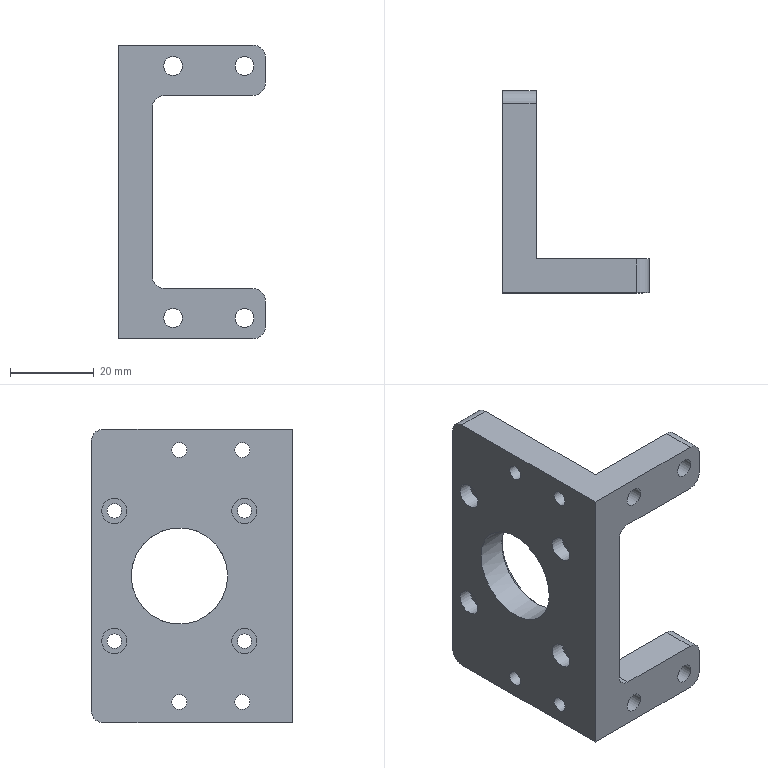CAM job | NX | 3+2 milling, drilling | part box 35 x 48 x 70 mm | stock box 40 x 53 x 75 mm
Tools:
number,name,description,diameter,corner_radius,flute_length,length,flutes
4,D4,平底铣刀-粗,4.0,0.0,25.0,75.0,2
9,D10,平底铣刀-粗,10.0,0.0,35.0,75.0,2
11,D4-J,平底铣刀-精,4.0,0.0,50.0,75.0,2
10,D10-J,平底铣刀-精,10.0,0.0,35.0,75.0,2
1,D80R0.8飞刀,圆鼻刀-粗,80.0,0.8,50.0,75.0,2
18,D6R0.5-J,圆鼻刀-精,6.0,0.5,50.0,75.0,2
1,D80R0.8飞刀-J,圆鼻刀-精,80.0,0.8,50.0,75.0,2
2,D6倒角刀,倒角刀,6.0,0.0,3.0,25.0,2
13,ZT3.4,钻头,3.4,0.0,35.0,50.0,2
17,ZT3.6,钻头,3.6,0.0,35.0,50.0,2
18,ZT12,钻头,12.0,0.0,35.0,50.0,2
Operations:
program,operation,operation_type,tool,method,geometry_group,spindle_rpm,surface_speed,feed_per_tooth,feed_cut,feed_plunge,cut_length_mm,path_length_mm,cut_time_min,machine_time_min
B,底壁铣飞面一刀开粗_COPY,VolumeBased25DMillingOperation,D80R0.8飞刀,分层开粗-切深K-步距G,W-B,2800.0,703.696,0.5357,3000.0,100.0,1603.746,3195.967,0.5346,0.6938
B,底壁铣飞面一刀精光_COPY,VolumeBased25DMillingOperation,D80R0.8飞刀-J,侧刃精光-切深K-步距G,W-B,4000.0,1005.28,0.125,1000.0,100.0,177.998,213.998,0.178,0.1816
B,型腔铣开粗-中_COPY,CavityMilling,D10,分层开粗-切深K-步距G,W-B,8000.0,251.327,0.2812,4500.0,100.0,35928.286,40055.198,7.984,8.536
B,铣沉头_1,CylinderMilling,D4,METHOD,W-B,8000.0,100.531,0.075,1200.0,100.0,467.722,946.122,0.3898,0.4376
B,铣孔_1,CylinderMilling,D4,METHOD,W-B,8000.0,100.531,0.0375,600.0,100.0,37.039,530.239,0.0617,0.1111
B,等高精光往复爬面_COPY,ZLevelMilling,D6R0.5-J,等高爬面-切深K-步距G,W-B,7000.0,131.947,0.3214,4500.0,100.0,2329.952,2545.794,0.5178,0.5394
B,钻倒角_2,Operation,D6倒角刀,METHOD,W-B,8000.0,150.796,0.0625,1000.0,0.0,20.0,236.435,0.02,0.0416
B,底壁铣倒角_COPY,VolumeBased25DMillingOperation,D6倒角刀,爬面_倒角-切深0-步距G,W-B,6500.0,122.519,0.1154,1500.0,100.0,292.022,386.423,0.1947,0.2041
B,底壁铣精光底面-中_COPY,VolumeBased25DMillingOperation,D10-J,精光步距切深关,W-B,7000.0,175.0,0.0536,1500.0,100.0,722.843,802.843,0.4819,0.4899
B,底壁铣精光侧面-中_COPY_1,VolumeBased25DMillingOperation,D10-J,侧刃精光-切深K-步距G,W-B,8000.0,251.32,0.0625,1000.0,100.0,132.265,387.447,0.1323,0.1578
B,底壁铣精光侧面-中-选底面_COPY,VolumeBased25DMillingOperation,D10-J,侧刃精光-切深K-步距G,W-B,8000.0,251.32,0.0625,1000.0,100.0,103.363,209.965,0.1034,0.114
B,底壁铣精光侧面-中_COPY_2,VolumeBased25DMillingOperation,D10-J,侧刃精光-切深K-步距G,W-B,8000.0,251.32,0.0625,1000.0,100.0,104.173,281.837,0.1042,0.1219
B,等高精光往复爬面_COPY_COPY,ZLevelMilling,D10-J,等高爬面-切深K-步距G,W-B,7000.0,131.947,0.3214,4500.0,100.0,5884.615,6081.864,1.308,1.327
B,平面去毛刺6X45L_COPY,SurfaceContour,D6倒角刀,爬面_倒角-切深0-步距G,W-B,6500.0,122.519,0.1154,1500.0,100.0,512.932,1354.344,0.342,0.4261
A,顶面开粗,FaceMilling,D80R0.8飞刀,分层开粗-切深K-步距G,W-A,4000.0,1005.31,0.375,3000.0,100.0,164.0,199.8,0.0547,0.0582
A,顶面,FaceMilling,D80R0.8飞刀,侧刃精光-切深K-步距G,W-A,4000.0,1005.31,0.125,1000.0,100.0,164.0,200.0,0.164,0.1676
A,外形粗_2,VolumeBased25DMillingOperation,D10,METHOD,W-A,8000.0,251.327,0.3125,5000.0,80.0,19646.241,19720.241,3.929,3.937
A,打点-深0.8,Operation,D6倒角刀,NONE,W-A,8000.0,150.796,0.0312,500.0,90.0,16.2,225.936,0.0324,0.0534
A,沉头孔-钻孔0段,Operation,ZT3.4,NONE,W-A,2800.0,29.908,0.0179,100.0,90.0,48.086,232.22,0.4809,0.4993
A,通孔-3-4,Operation,ZT3.6,NONE,W-A,3000.0,33.929,0.02,120.0,90.0,52.0,237.075,0.4333,0.4518
A,通孔-12.5-25,Operation,ZT12,NONE,W-A,800.0,30.159,0.125,200.0,90.0,14.605,69.21,0.073,0.0785
A,铣孔开粗D8_1,CylinderMilling,D10,NONE,W-A,8000.0,201.062,0.075,1200.0,100.0,784.197,832.197,0.6535,0.6583
A,铣孔开粗D4_1,CylinderMilling,D4,NONE,W-A,8000.0,100.531,0.075,1200.0,100.0,328.396,592.996,0.2737,0.3001
A,铣孔精光D4_1,CylinderMilling,D4-J,精光步距切深关,W-A,8000.0,100.531,0.0312,500.0,100.0,62.334,326.934,0.1247,0.1511
A,仅选体,SurfaceContour,D6倒角刀,METHOD,W-A,8000.0,150.796,0.1875,3000.0,100.0,324.025,426.376,0.108,0.1182
A,钻倒角_1,Operation,D6倒角刀,METHOD,W-A,8000.0,150.796,0.0312,500.0,0.0,20.4,180.469,0.0408,0.0568
A,铣倒角_1,PlanarMilling,D6倒角刀,NONE,W-A,8000.0,150.796,0.0312,500.0,100.0,110.739,349.474,0.2215,0.2454
A,铣倒角_2,PlanarMilling,D6倒角刀,METHOD,W-A,8000.0,150.796,0.0625,1000.0,100.0,75.142,117.142,0.0751,0.0793
A,外形半精_2,VolumeBased25DMillingOperation,D10-J,METHOD,W-A,8000.0,251.327,0.0625,1000.0,100.0,809.397,1072.626,0.8094,0.8357
A,底壁铣精光侧面-中_COPY,VolumeBased25DMillingOperation,D10-J,侧刃精光-切深K-步距G,W-A,8000.0,251.32,0.0625,1000.0,100.0,49.814,82.214,0.0498,0.0531